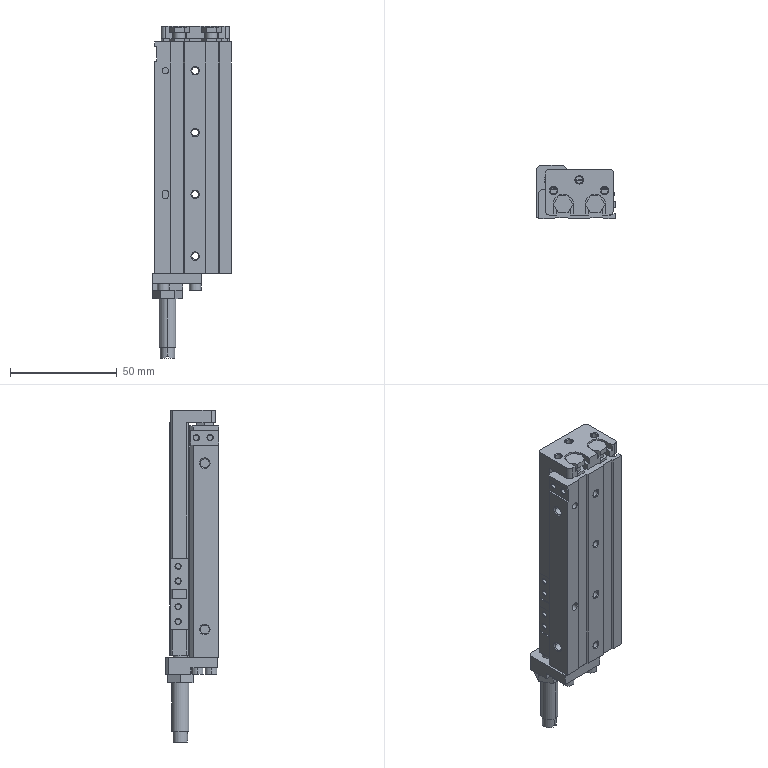Part | STEP file | MXQ8-50BT | 3 solids | 425 faces | box 37 x 25 x 155.8 mm | volume 80767 mm3 | plane 224 | cylinder 143 | cone 58 | commonest cylinder face diameters 2.459 x40 3.242 x14 4 x14 6.5 x10 8 x10 3 x8